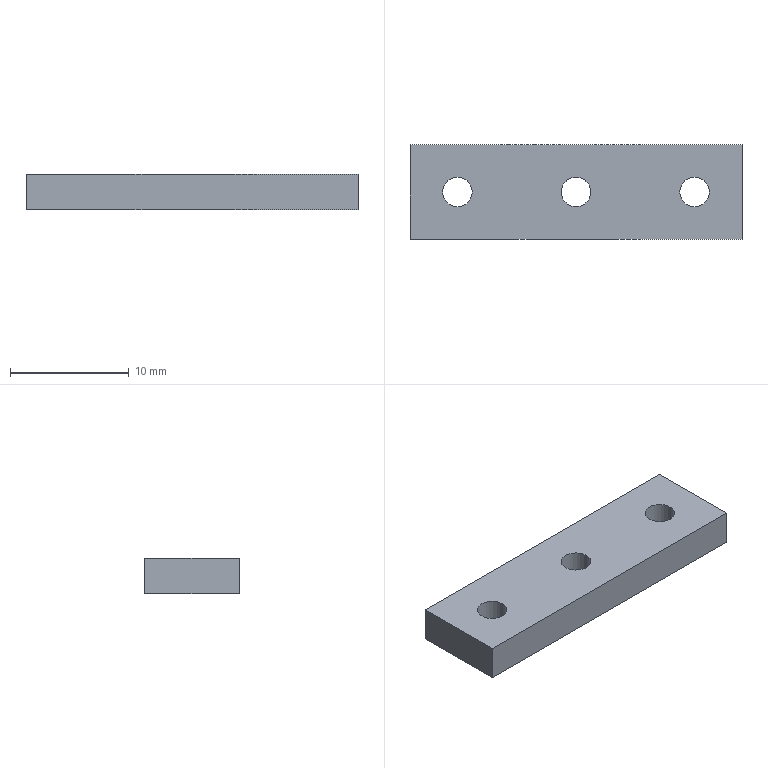Part | SolidWorks | features 3DProfileFeature 2, HoleWzd 2, Extrusion 1 | 1 solid | 12 faces | box 28 x 8 x 3 mm | volume 627.821 mm3 | cylinder 6 | plane 6 | commonest cylinder face diameters 2.5 x6
STEP:
#1=CARTESIAN_POINT('',(12.75,-4.,0.));
#2=VERTEX_POINT('',#1);
#3=CARTESIAN_POINT('',(15.25,-4.,0.));
#4=VERTEX_POINT('',#3);
#5=CARTESIAN_POINT('',(14.,-4.,0.));
#6=DIRECTION('',(0.,0.,1.));
#7=DIRECTION('',(1.,0.,0.));
#8=AXIS2_PLACEMENT_3D('',#5,#6,#7);
#9=CIRCLE('',#8,1.25);
#10=EDGE_CURVE('',#2,#4,#9,.T.);
#11=ORIENTED_EDGE('',*,*,#10,.F.);
#12=CARTESIAN_POINT('',(12.75,-4.,3.));
#13=VERTEX_POINT('',#12);
#14=CARTESIAN_POINT('',(12.75,-4.,3.));
#15=DIRECTION('',(0.,0.,1.));
#16=VECTOR('',#15,1000.);
#17=LINE('',#14,#16);
#18=EDGE_CURVE('',#2,#13,#17,.T.);
#19=ORIENTED_EDGE('',*,*,#18,.T.);
#20=CARTESIAN_POINT('',(15.25,-4.,3.));
#21=VERTEX_POINT('',#20);
#22=CARTESIAN_POINT('',(14.,-4.,3.));
#23=DIRECTION('',(0.,0.,1.));
#24=DIRECTION('',(1.,0.,0.));
#25=AXIS2_PLACEMENT_3D('',#22,#23,#24);
#26=CIRCLE('',#25,1.25);
#27=EDGE_CURVE('',#13,#21,#26,.T.);
#28=ORIENTED_EDGE('',*,*,#27,.T.);
#29=CARTESIAN_POINT('',(15.25,-4.,3.));
#30=DIRECTION('',(0.,0.,1.));
#31=VECTOR('',#30,1000.);
#32=LINE('',#29,#31);
#33=EDGE_CURVE('',#4,#21,#32,.T.);
#34=ORIENTED_EDGE('',*,*,#33,.F.);
#35=EDGE_LOOP('',(#11,#19,#28,#34));
#36=FACE_OUTER_BOUND('',#35,.T.);
#37=CARTESIAN_POINT('',(14.,-4.,3.));
#38=DIRECTION('',(0.,0.,1.));
#39=DIRECTION('',(1.,0.,0.));
#40=AXIS2_PLACEMENT_3D('',#37,#38,#39);
#41=CYLINDRICAL_SURFACE('',#40,1.25);
#42=ADVANCED_FACE('',(#36),#41,.F.);
#43=CARTESIAN_POINT('',(22.75,-4.,3.));
#44=VERTEX_POINT('',#43);
#45=CARTESIAN_POINT('',(25.25,-4.,3.));
#46=VERTEX_POINT('',#45);
#47=CARTESIAN_POINT('',(24.,-4.,3.));
#48=DIRECTION('',(0.,0.,1.));
#49=DIRECTION('',(-1.,0.,0.));
#50=AXIS2_PLACEMENT_3D('',#47,#48,#49);
#51=CIRCLE('',#50,1.25);
#52=EDGE_CURVE('',#44,#46,#51,.T.);
#53=ORIENTED_EDGE('',*,*,#52,.T.);
#54=CARTESIAN_POINT('',(25.25,-4.,0.));
#55=VERTEX_POINT('',#54);
#56=CARTESIAN_POINT('',(25.25,-4.,3.));
#57=DIRECTION('',(0.,0.,-1.));
#58=VECTOR('',#57,1000.);
#59=LINE('',#56,#58);
#60=EDGE_CURVE('',#46,#55,#59,.T.);
#61=ORIENTED_EDGE('',*,*,#60,.T.);
#62=CARTESIAN_POINT('',(22.75,-4.,0.));
#63=VERTEX_POINT('',#62);
#64=CARTESIAN_POINT('',(24.,-4.,0.));
#65=DIRECTION('',(0.,0.,1.));
#66=DIRECTION('',(-1.,0.,0.));
#67=AXIS2_PLACEMENT_3D('',#64,#65,#66);
#68=CIRCLE('',#67,1.25);
#69=EDGE_CURVE('',#63,#55,#68,.T.);
#70=ORIENTED_EDGE('',*,*,#69,.F.);
#71=CARTESIAN_POINT('',(22.75,-4.,3.));
#72=DIRECTION('',(0.,0.,-1.));
#73=VECTOR('',#72,1000.);
#74=LINE('',#71,#73);
#75=EDGE_CURVE('',#44,#63,#74,.T.);
#76=ORIENTED_EDGE('',*,*,#75,.F.);
#77=EDGE_LOOP('',(#53,#61,#70,#76));
#78=FACE_OUTER_BOUND('',#77,.T.);
#79=CARTESIAN_POINT('',(24.,-4.,3.));
#80=DIRECTION('',(0.,0.,-1.));
#81=DIRECTION('',(-1.,0.,0.));
#82=AXIS2_PLACEMENT_3D('',#79,#80,#81);
#83=CYLINDRICAL_SURFACE('',#82,1.25);
#84=ADVANCED_FACE('',(#78),#83,.F.);
#85=CARTESIAN_POINT('',(2.75,-4.,3.));
#86=VERTEX_POINT('',#85);
#87=CARTESIAN_POINT('',(5.25,-4.,3.));
#88=VERTEX_POINT('',#87);
#89=CARTESIAN_POINT('',(4.,-4.,3.));
#90=DIRECTION('',(0.,0.,1.));
#91=DIRECTION('',(1.,0.,0.));
#92=AXIS2_PLACEMENT_3D('',#89,#90,#91);
#93=CIRCLE('',#92,1.25);
#94=EDGE_CURVE('',#86,#88,#93,.T.);
#95=ORIENTED_EDGE('',*,*,#94,.T.);
#96=CARTESIAN_POINT('',(5.25,-4.,0.));
#97=VERTEX_POINT('',#96);
#98=CARTESIAN_POINT('',(5.25,-4.,3.));
#99=DIRECTION('',(0.,0.,-1.));
#100=VECTOR('',#99,1000.);
#101=LINE('',#98,#100);
#102=EDGE_CURVE('',#88,#97,#101,.T.);
#103=ORIENTED_EDGE('',*,*,#102,.T.);
#104=CARTESIAN_POINT('',(2.75,-4.,0.));
#105=VERTEX_POINT('',#104);
#106=CARTESIAN_POINT('',(4.,-4.,0.));
#107=DIRECTION('',(0.,0.,1.));
#108=DIRECTION('',(1.,0.,0.));
#109=AXIS2_PLACEMENT_3D('',#106,#107,#108);
#110=CIRCLE('',#109,1.25);
#111=EDGE_CURVE('',#105,#97,#110,.T.);
#112=ORIENTED_EDGE('',*,*,#111,.F.);
#113=CARTESIAN_POINT('',(2.75,-4.,3.));
#114=DIRECTION('',(0.,0.,-1.));
#115=VECTOR('',#114,1000.);
#116=LINE('',#113,#115);
#117=EDGE_CURVE('',#86,#105,#116,.T.);
#118=ORIENTED_EDGE('',*,*,#117,.F.);
#119=EDGE_LOOP('',(#95,#103,#112,#118));
#120=FACE_OUTER_BOUND('',#119,.T.);
#121=CARTESIAN_POINT('',(4.,-4.,3.));
#122=DIRECTION('',(0.,0.,-1.));
#123=DIRECTION('',(-1.,0.,0.));
#124=AXIS2_PLACEMENT_3D('',#121,#122,#123);
#125=CYLINDRICAL_SURFACE('',#124,1.25);
#126=ADVANCED_FACE('',(#120),#125,.F.);
#127=CARTESIAN_POINT('',(14.,-4.,3.));
#128=DIRECTION('',(0.,0.,1.));
#129=DIRECTION('',(1.,0.,0.));
#130=AXIS2_PLACEMENT_3D('',#127,#128,#129);
#131=CIRCLE('',#130,1.25);
#132=EDGE_CURVE('',#21,#13,#131,.T.);
#133=ORIENTED_EDGE('',*,*,#132,.F.);
#134=ORIENTED_EDGE('',*,*,#27,.F.);
#135=EDGE_LOOP('',(#133,#134));
#136=FACE_BOUND('',#135,.T.);
#137=ORIENTED_EDGE('',*,*,#94,.F.);
#138=CARTESIAN_POINT('',(4.,-4.,3.));
#139=DIRECTION('',(0.,0.,1.));
#140=DIRECTION('',(1.,0.,0.));
#141=AXIS2_PLACEMENT_3D('',#138,#139,#140);
#142=CIRCLE('',#141,1.25);
#143=EDGE_CURVE('',#88,#86,#142,.T.);
#144=ORIENTED_EDGE('',*,*,#143,.F.);
#145=EDGE_LOOP('',(#137,#144));
#146=FACE_BOUND('',#145,.T.);
#147=CARTESIAN_POINT('',(0.,0.,3.));
#148=VERTEX_POINT('',#147);
#149=CARTESIAN_POINT('',(0.,-8.,3.));
#150=VERTEX_POINT('',#149);
#151=CARTESIAN_POINT('',(0.,0.,3.));
#152=DIRECTION('',(0.,-1.,0.));
#153=VECTOR('',#152,1000.);
#154=LINE('',#151,#153);
#155=EDGE_CURVE('',#148,#150,#154,.T.);
#156=ORIENTED_EDGE('',*,*,#155,.T.);
#157=CARTESIAN_POINT('',(28.,-8.,3.));
#158=VERTEX_POINT('',#157);
#159=CARTESIAN_POINT('',(0.,-8.,3.));
#160=DIRECTION('',(1.,0.,0.));
#161=VECTOR('',#160,1000.);
#162=LINE('',#159,#161);
#163=EDGE_CURVE('',#150,#158,#162,.T.);
#164=ORIENTED_EDGE('',*,*,#163,.T.);
#165=CARTESIAN_POINT('',(28.,0.,3.));
#166=VERTEX_POINT('',#165);
#167=CARTESIAN_POINT('',(28.,0.,3.));
#168=DIRECTION('',(0.,1.,0.));
#169=VECTOR('',#168,1000.);
#170=LINE('',#167,#169);
#171=EDGE_CURVE('',#158,#166,#170,.T.);
#172=ORIENTED_EDGE('',*,*,#171,.T.);
#173=CARTESIAN_POINT('',(0.,0.,3.));
#174=DIRECTION('',(-1.,0.,0.));
#175=VECTOR('',#174,1000.);
#176=LINE('',#173,#175);
#177=EDGE_CURVE('',#166,#148,#176,.T.);
#178=ORIENTED_EDGE('',*,*,#177,.T.);
#179=EDGE_LOOP('',(#156,#164,#172,#178));
#180=FACE_OUTER_BOUND('',#179,.T.);
#181=ORIENTED_EDGE('',*,*,#52,.F.);
#182=CARTESIAN_POINT('',(24.,-4.,3.));
#183=DIRECTION('',(0.,0.,1.));
#184=DIRECTION('',(-1.,0.,0.));
#185=AXIS2_PLACEMENT_3D('',#182,#183,#184);
#186=CIRCLE('',#185,1.25);
#187=EDGE_CURVE('',#46,#44,#186,.T.);
#188=ORIENTED_EDGE('',*,*,#187,.F.);
#189=EDGE_LOOP('',(#181,#188));
#190=FACE_BOUND('',#189,.T.);
#191=CARTESIAN_POINT('',(0.,0.,3.));
#192=DIRECTION('',(0.,0.,1.));
#193=DIRECTION('',(1.,0.,0.));
#194=AXIS2_PLACEMENT_3D('',#191,#192,#193);
#195=PLANE('',#194);
#196=ADVANCED_FACE('',(#136,#146,#180,#190),#195,.T.);
#197=CARTESIAN_POINT('',(14.,-4.,0.));
#198=DIRECTION('',(0.,0.,1.));
#199=DIRECTION('',(1.,0.,0.));
#200=AXIS2_PLACEMENT_3D('',#197,#198,#199);
#201=CIRCLE('',#200,1.25);
#202=EDGE_CURVE('',#4,#2,#201,.T.);
#203=ORIENTED_EDGE('',*,*,#202,.T.);
#204=ORIENTED_EDGE('',*,*,#10,.T.);
#205=EDGE_LOOP('',(#203,#204));
#206=FACE_BOUND('',#205,.T.);
#207=CARTESIAN_POINT('',(0.,0.,0.));
#208=VERTEX_POINT('',#207);
#209=CARTESIAN_POINT('',(0.,-8.,0.));
#210=VERTEX_POINT('',#209);
#211=CARTESIAN_POINT('',(0.,0.,0.));
#212=DIRECTION('',(0.,-1.,0.));
#213=VECTOR('',#212,1000.);
#214=LINE('',#211,#213);
#215=EDGE_CURVE('',#208,#210,#214,.T.);
#216=ORIENTED_EDGE('',*,*,#215,.F.);
#217=CARTESIAN_POINT('',(28.,0.,0.));
#218=VERTEX_POINT('',#217);
#219=CARTESIAN_POINT('',(0.,0.,0.));
#220=DIRECTION('',(-1.,0.,0.));
#221=VECTOR('',#220,1000.);
#222=LINE('',#219,#221);
#223=EDGE_CURVE('',#218,#208,#222,.T.);
#224=ORIENTED_EDGE('',*,*,#223,.F.);
#225=CARTESIAN_POINT('',(28.,-8.,0.));
#226=VERTEX_POINT('',#225);
#227=CARTESIAN_POINT('',(28.,0.,0.));
#228=DIRECTION('',(0.,1.,0.));
#229=VECTOR('',#228,1000.);
#230=LINE('',#227,#229);
#231=EDGE_CURVE('',#226,#218,#230,.T.);
#232=ORIENTED_EDGE('',*,*,#231,.F.);
#233=CARTESIAN_POINT('',(0.,-8.,0.));
#234=DIRECTION('',(1.,0.,0.));
#235=VECTOR('',#234,1000.);
#236=LINE('',#233,#235);
#237=EDGE_CURVE('',#210,#226,#236,.T.);
#238=ORIENTED_EDGE('',*,*,#237,.F.);
#239=EDGE_LOOP('',(#216,#224,#232,#238));
#240=FACE_OUTER_BOUND('',#239,.T.);
#241=ORIENTED_EDGE('',*,*,#111,.T.);
#242=CARTESIAN_POINT('',(4.,-4.,0.));
#243=DIRECTION('',(0.,0.,1.));
#244=DIRECTION('',(1.,0.,0.));
#245=AXIS2_PLACEMENT_3D('',#242,#243,#244);
#246=CIRCLE('',#245,1.25);
#247=EDGE_CURVE('',#97,#105,#246,.T.);
#248=ORIENTED_EDGE('',*,*,#247,.T.);
#249=EDGE_LOOP('',(#241,#248));
#250=FACE_BOUND('',#249,.T.);
#251=ORIENTED_EDGE('',*,*,#69,.T.);
#252=CARTESIAN_POINT('',(24.,-4.,0.));
#253=DIRECTION('',(0.,0.,1.));
#254=DIRECTION('',(-1.,0.,0.));
#255=AXIS2_PLACEMENT_3D('',#252,#253,#254);
#256=CIRCLE('',#255,1.25);
#257=EDGE_CURVE('',#55,#63,#256,.T.);
#258=ORIENTED_EDGE('',*,*,#257,.T.);
#259=EDGE_LOOP('',(#251,#258));
#260=FACE_BOUND('',#259,.T.);
#261=CARTESIAN_POINT('',(0.,0.,0.));
#262=DIRECTION('',(0.,0.,1.));
#263=DIRECTION('',(1.,0.,0.));
#264=AXIS2_PLACEMENT_3D('',#261,#262,#263);
#265=PLANE('',#264);
#266=ADVANCED_FACE('',(#206,#240,#250,#260),#265,.F.);
#267=ORIENTED_EDGE('',*,*,#215,.T.);
#268=CARTESIAN_POINT('',(0.,-8.,3.));
#269=DIRECTION('',(0.,0.,-1.));
#270=VECTOR('',#269,1000.);
#271=LINE('',#268,#270);
#272=EDGE_CURVE('',#150,#210,#271,.T.);
#273=ORIENTED_EDGE('',*,*,#272,.F.);
#274=ORIENTED_EDGE('',*,*,#155,.F.);
#275=CARTESIAN_POINT('',(0.,0.,3.));
#276=DIRECTION('',(0.,0.,-1.));
#277=VECTOR('',#276,1000.);
#278=LINE('',#275,#277);
#279=EDGE_CURVE('',#148,#208,#278,.T.);
#280=ORIENTED_EDGE('',*,*,#279,.T.);
#281=EDGE_LOOP('',(#267,#273,#274,#280));
#282=FACE_OUTER_BOUND('',#281,.T.);
#283=CARTESIAN_POINT('',(0.,0.,3.));
#284=DIRECTION('',(1.,0.,0.));
#285=DIRECTION('',(0.,1.,0.));
#286=AXIS2_PLACEMENT_3D('',#283,#284,#285);
#287=PLANE('',#286);
#288=ADVANCED_FACE('',(#282),#287,.F.);
#289=ORIENTED_EDGE('',*,*,#237,.T.);
#290=CARTESIAN_POINT('',(28.,-8.,3.));
#291=DIRECTION('',(0.,0.,-1.));
#292=VECTOR('',#291,1000.);
#293=LINE('',#290,#292);
#294=EDGE_CURVE('',#158,#226,#293,.T.);
#295=ORIENTED_EDGE('',*,*,#294,.F.);
#296=ORIENTED_EDGE('',*,*,#163,.F.);
#297=ORIENTED_EDGE('',*,*,#272,.T.);
#298=EDGE_LOOP('',(#289,#295,#296,#297));
#299=FACE_OUTER_BOUND('',#298,.T.);
#300=CARTESIAN_POINT('',(0.,-8.,3.));
#301=DIRECTION('',(0.,1.,0.));
#302=DIRECTION('',(0.,0.,1.));
#303=AXIS2_PLACEMENT_3D('',#300,#301,#302);
#304=PLANE('',#303);
#305=ADVANCED_FACE('',(#299),#304,.F.);
#306=ORIENTED_EDGE('',*,*,#231,.T.);
#307=CARTESIAN_POINT('',(28.,0.,3.));
#308=DIRECTION('',(0.,0.,-1.));
#309=VECTOR('',#308,1000.);
#310=LINE('',#307,#309);
#311=EDGE_CURVE('',#166,#218,#310,.T.);
#312=ORIENTED_EDGE('',*,*,#311,.F.);
#313=ORIENTED_EDGE('',*,*,#171,.F.);
#314=ORIENTED_EDGE('',*,*,#294,.T.);
#315=EDGE_LOOP('',(#306,#312,#313,#314));
#316=FACE_OUTER_BOUND('',#315,.T.);
#317=CARTESIAN_POINT('',(28.,0.,3.));
#318=DIRECTION('',(-1.,0.,0.));
#319=DIRECTION('',(0.,0.,1.));
#320=AXIS2_PLACEMENT_3D('',#317,#318,#319);
#321=PLANE('',#320);
#322=ADVANCED_FACE('',(#316),#321,.F.);
#323=ORIENTED_EDGE('',*,*,#223,.T.);
#324=ORIENTED_EDGE('',*,*,#279,.F.);
#325=ORIENTED_EDGE('',*,*,#177,.F.);
#326=ORIENTED_EDGE('',*,*,#311,.T.);
#327=EDGE_LOOP('',(#323,#324,#325,#326));
#328=FACE_OUTER_BOUND('',#327,.T.);
#329=CARTESIAN_POINT('',(0.,0.,3.));
#330=DIRECTION('',(0.,-1.,0.));
#331=DIRECTION('',(0.,0.,-1.));
#332=AXIS2_PLACEMENT_3D('',#329,#330,#331);
#333=PLANE('',#332);
#334=ADVANCED_FACE('',(#328),#333,.F.);
#335=ORIENTED_EDGE('',*,*,#102,.F.);
#336=ORIENTED_EDGE('',*,*,#143,.T.);
#337=ORIENTED_EDGE('',*,*,#117,.T.);
#338=ORIENTED_EDGE('',*,*,#247,.F.);
#339=EDGE_LOOP('',(#335,#336,#337,#338));
#340=FACE_OUTER_BOUND('',#339,.T.);
#341=CARTESIAN_POINT('',(4.,-4.,3.));
#342=DIRECTION('',(0.,0.,-1.));
#343=DIRECTION('',(-1.,0.,0.));
#344=AXIS2_PLACEMENT_3D('',#341,#342,#343);
#345=CYLINDRICAL_SURFACE('',#344,1.25);
#346=ADVANCED_FACE('',(#340),#345,.F.);
#347=ORIENTED_EDGE('',*,*,#60,.F.);
#348=ORIENTED_EDGE('',*,*,#187,.T.);
#349=ORIENTED_EDGE('',*,*,#75,.T.);
#350=ORIENTED_EDGE('',*,*,#257,.F.);
#351=EDGE_LOOP('',(#347,#348,#349,#350));
#352=FACE_OUTER_BOUND('',#351,.T.);
#353=CARTESIAN_POINT('',(24.,-4.,3.));
#354=DIRECTION('',(0.,0.,-1.));
#355=DIRECTION('',(-1.,0.,0.));
#356=AXIS2_PLACEMENT_3D('',#353,#354,#355);
#357=CYLINDRICAL_SURFACE('',#356,1.25);
#358=ADVANCED_FACE('',(#352),#357,.F.);
#359=ORIENTED_EDGE('',*,*,#18,.F.);
#360=ORIENTED_EDGE('',*,*,#202,.F.);
#361=ORIENTED_EDGE('',*,*,#33,.T.);
#362=ORIENTED_EDGE('',*,*,#132,.T.);
#363=EDGE_LOOP('',(#359,#360,#361,#362));
#364=FACE_OUTER_BOUND('',#363,.T.);
#365=CARTESIAN_POINT('',(14.,-4.,3.));
#366=DIRECTION('',(0.,0.,1.));
#367=DIRECTION('',(1.,0.,0.));
#368=AXIS2_PLACEMENT_3D('',#365,#366,#367);
#369=CYLINDRICAL_SURFACE('',#368,1.25);
#370=ADVANCED_FACE('',(#364),#369,.F.);
#371=CLOSED_SHELL('',(#42,#84,#126,#196,#266,#288,#305,#322,#334,#346,#358,#370));
#372=MANIFOLD_SOLID_BREP('',#371);
#373=CARTESIAN_POINT('',(0.,0.,0.));
#374=DIRECTION('',(0.,0.,1.));
#375=DIRECTION('',(1.,0.,0.));
#376=AXIS2_PLACEMENT_3D('',#373,#374,#375);
#377=(LENGTH_UNIT()NAMED_UNIT(*)SI_UNIT(.MILLI.,.METRE.));
#378=UNCERTAINTY_MEASURE_WITH_UNIT(LENGTH_MEASURE(0.00001),#377,'','');
#379=(NAMED_UNIT(*)PLANE_ANGLE_UNIT()SI_UNIT($,.RADIAN.));
#380=(NAMED_UNIT(*)SI_UNIT($,.STERADIAN.)SOLID_ANGLE_UNIT());
#381=(GEOMETRIC_REPRESENTATION_CONTEXT(3)GLOBAL_UNCERTAINTY_ASSIGNED_CONTEXT((#378))GLOBAL_UNIT_ASSIGNED_CONTEXT((#377,#379,#380))REPRESENTATION_CONTEXT('',''));
#382=ADVANCED_BREP_SHAPE_REPRESENTATION('',(#372,#376),#381);